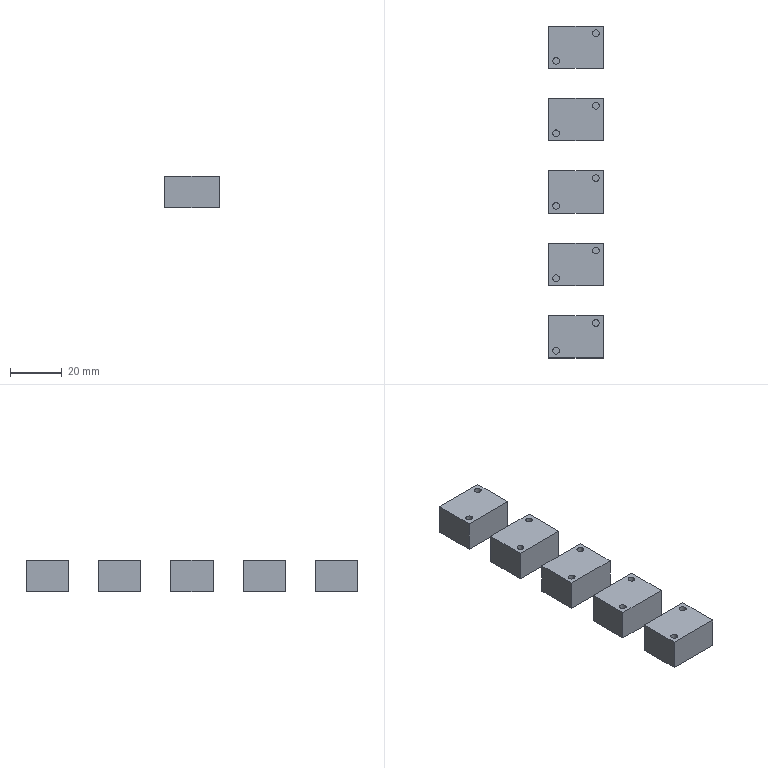NC program | NX | posted with a generic post | part box 21 x 128.262 x 12 mm
Lines 3118 to 3295 of 3295:
(PLANAR_MILL , TOOL : D6A45)
N6210 T07 M6
N6212 G54
N6214 G17 G0 G90 X61.684 Y-7.911 S9500 M3
N6216 G43 Z30. H7
N6218 Z0.5
N6220 G94 G1 Z-1. F1250.
N6222 G3 X61.731 Y-7.7 R0.5
N6224 X61.331 Y-7.3 R0.4
N6226 X61.731 Y-7.7 R-0.4
N6228 X61.684 Y-7.489 R0.5
N6230 G1 Z0.5
N6232 G0 Z30.
N6234 X65.388 Y0.766
N6236 Z0.5
N6238 G1 Z-1.
N6240 G3 X65.031 Y0. R1.
N6242 G1 Y-10.5
N6244 G2 X64.131 Y-11.4 R0.9
N6246 G1 X47.869
N6248 G2 X46.969 Y-10.5 R0.9
N6250 G1 Y10.5
N6252 G2 X47.869 Y11.4 R0.9
N6254 G1 X64.131
N6256 G2 X65.031 Y10.5 R0.9
N6258 G1 Y0.
N6260 G3 X65.388 Y-0.766 R1.
N6262 G1 Z0.5
N6264 G0 Z30.
N6266 X50.88 Y8.053
N6268 Z0.5
N6270 G1 Z-1.
N6272 G3 X50.669 Y8.1 R0.5
N6274 X50.269 Y7.7 R0.4
N6276 X50.669 Y8.1 R-0.4
N6278 X50.457 Y8.053 R0.5
N6280 G1 Z0.5
N6282 G0 Z30.
N6284 X33.12 Y-8.053
N6286 Z0.5
N6288 G1 Z-1.
N6290 G3 X33.331 Y-8.1 R0.5
N6292 X33.731 Y-7.7 R0.4
N6294 X33.331 Y-8.1 R-0.4
N6296 X33.543 Y-8.053 R0.5
N6298 G1 Z0.5
N6300 G0 Z30.
N6302 X37.388 Y0.766
N6304 Z0.5
N6306 G1 Z-1.
N6308 G3 X37.031 Y0. R1.
N6310 G1 Y-10.5
N6312 G2 X36.131 Y-11.4 R0.9
N6314 G1 X19.869
N6316 G2 X18.969 Y-10.5 R0.9
N6318 G1 Y10.5
N6320 G2 X19.869 Y11.4 R0.9
N6322 G1 X36.131
N6324 G2 X37.031 Y10.5 R0.9
N6326 G1 Y0.
N6328 G3 X37.388 Y-0.766 R1.
N6330 G1 Z0.5
N6332 G0 Z30.
N6334 X22.88 Y8.053
N6336 Z0.5
N6338 G1 Z-1.
N6340 G3 X22.669 Y8.1 R0.5
N6342 X22.269 Y7.7 R0.4
N6344 X22.669 Y8.1 R-0.4
N6346 X22.457 Y8.053 R0.5
N6348 G1 Z0.5
N6350 G0 Z30.
N6352 X5.12 Y-8.053
N6354 Z0.5
N6356 G1 Z-1.
N6358 G3 X5.331 Y-8.1 R0.5
N6360 X5.731 Y-7.7 R0.4
N6362 X5.331 Y-8.1 R-0.4
N6364 X5.543 Y-8.053 R0.5
N6366 G1 Z0.5
N6368 G0 Z30.
N6370 X9.388 Y0.766
N6372 Z0.5
N6374 G1 Z-1.
N6376 G3 X9.031 Y0. R1.
N6378 G1 Y-10.5
N6380 G2 X8.131 Y-11.4 R0.9
N6382 G1 X-8.131
N6384 G2 X-9.031 Y-10.5 R0.9
N6386 G1 Y10.5
N6388 G2 X-8.131 Y11.4 R0.9
N6390 G1 X8.131
N6392 G2 X9.031 Y10.5 R0.9
N6394 G1 Y0.
N6396 G3 X9.388 Y-0.766 R1.
N6398 G1 Z0.5
N6400 G0 Z30.
N6402 X-5.12 Y8.053
N6404 Z0.5
N6406 G1 Z-1.
N6408 G3 X-5.331 Y8.1 R0.5
N6410 X-5.731 Y7.7 R0.4
N6412 X-5.331 Y8.1 R-0.4
N6414 X-5.543 Y8.053 R0.5
N6416 G1 Z0.5
N6418 G0 Z30.
N6420 X-22.88 Y-8.053
N6422 Z0.5
N6424 G1 Z-1.
N6426 G3 X-22.669 Y-8.1 R0.5
N6428 X-22.269 Y-7.7 R0.4
N6430 X-22.669 Y-8.1 R-0.4
N6432 X-22.457 Y-8.053 R0.5
N6434 G1 Z0.5
N6436 G0 Z30.
N6438 X-18.612 Y0.766
N6440 Z0.5
N6442 G1 Z-1.
N6444 G3 X-18.969 Y0. R1.
N6446 G1 Y-10.5
N6448 G2 X-19.869 Y-11.4 R0.9
N6450 G1 X-36.131
N6452 G2 X-37.031 Y-10.5 R0.9
N6454 G1 Y10.5
N6456 G2 X-36.131 Y11.4 R0.9
N6458 G1 X-19.869
N6460 G2 X-18.969 Y10.5 R0.9
N6462 G1 Y0.
N6464 G3 X-18.612 Y-0.766 R1.
N6466 G1 Z0.5
N6468 G0 Z30.
N6470 X-33.12 Y8.053
N6472 Z0.5
N6474 G1 Z-1.
N6476 G3 X-33.331 Y8.1 R0.5
N6478 X-33.731 Y7.7 R0.4
N6480 X-33.331 Y8.1 R-0.4
N6482 X-33.543 Y8.053 R0.5
N6484 G1 Z0.5
N6486 G0 Z30.
N6488 X-50.88 Y-8.053
N6490 Z0.5
N6492 G1 Z-1.
N6494 G3 X-50.669 Y-8.1 R0.5
N6496 X-50.269 Y-7.7 R0.4
N6498 X-50.669 Y-8.1 R-0.4
N6500 X-50.457 Y-8.053 R0.5
N6502 G1 Z0.5
N6504 G0 Z30.
N6506 X-65.388 Y-0.766
N6508 Z0.5
N6510 G1 Z-1.
N6512 G3 X-65.031 Y0. R1.
N6514 G1 Y10.5
N6516 G2 X-64.131 Y11.4 R0.9
N6518 G1 X-47.869
N6520 G2 X-46.969 Y10.5 R0.9
N6522 G1 Y-10.5
N6524 G2 X-47.869 Y-11.4 R0.9
N6526 G1 X-64.131
N6528 G2 X-65.031 Y-10.5 R0.9
N6530 G1 Y0.
N6532 G3 X-65.388 Y0.766 R1.
N6534 G1 Z0.5
N6536 G0 Z30.
N6538 X-61.12 Y8.053
N6540 Z0.5
N6542 G1 Z-1.
N6544 G3 X-61.331 Y8.1 R0.5
N6546 X-61.731 Y7.7 R0.4
N6548 X-61.331 Y8.1 R-0.4
N6550 X-61.543 Y8.053 R0.5
N6552 G1 Z0.5
N6554 G0 Z30.
N6556 M5
N6558 M2